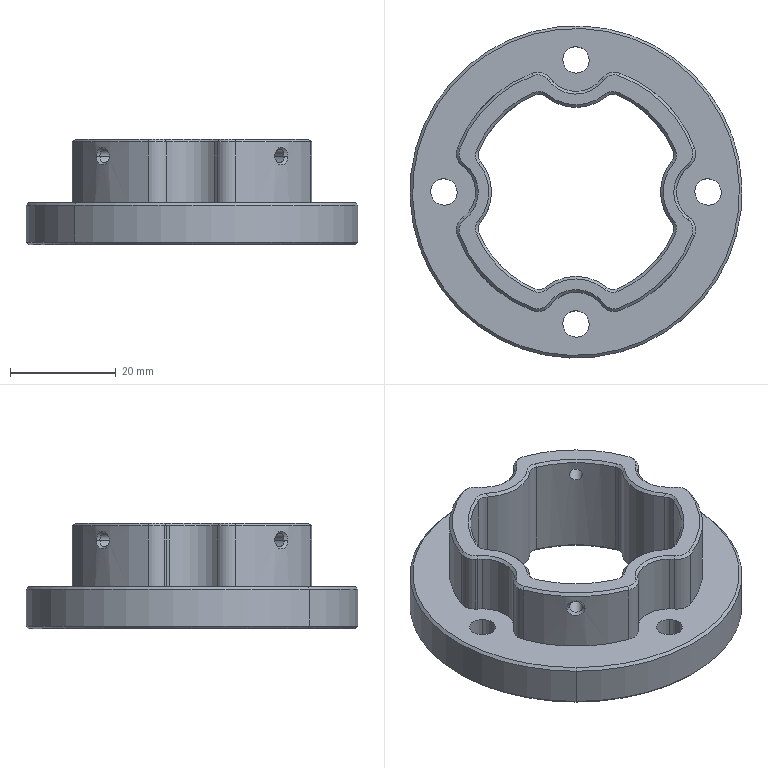Part | 1 solid | 126 faces | box 62.9 x 62.9 x 20 mm | volume 21460 mm3 | cone 59 | cylinder 56 | spline 8 | plane 3 | commonest cylinder face diameters 6 x10 2.5 x8 4 x8 5 x8 12 x6 39.9 x5